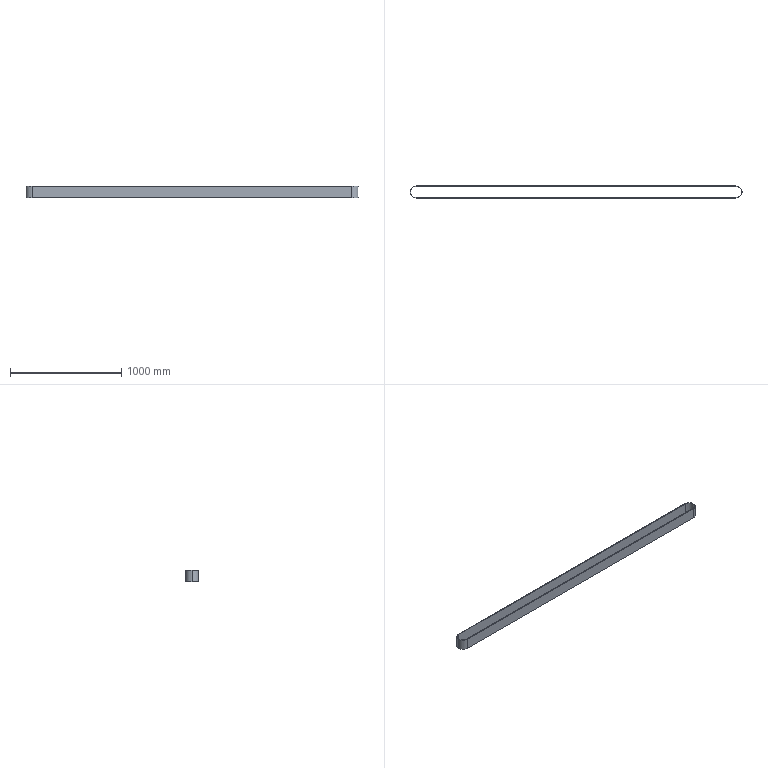Part | STEP file | 1 solid | 12 faces | box 2985 x 110 x 100 mm | volume 3039827 mm3 | cylinder 6 | plane 6 | commonest cylinder face diameters 100 x3 110 x3
STEP:
#1=CARTESIAN_POINT('',(0.,0.,0.));
#2=DIRECTION('',(0.,0.,1.));
#3=DIRECTION('',(1.,0.,0.));
#4=AXIS2_PLACEMENT_3D('',#1,#2,#3);
#5=CARTESIAN_POINT('',(-2874.893,50.,50.));
#6=VERTEX_POINT('',#5);
#7=CARTESIAN_POINT('',(-2874.893,50.,-50.));
#8=VERTEX_POINT('',#7);
#9=CARTESIAN_POINT('',(-2874.893,50.,50.));
#10=DIRECTION('',(0.,0.,-1.));
#11=VECTOR('',#10,1.);
#12=LINE('',#9,#11);
#13=CARTESIAN_POINT('',(-2874.893,0.,50.));
#14=DIRECTION('',(0.,0.,-1.));
#15=DIRECTION('',(-1.,0.,0.));
#16=AXIS2_PLACEMENT_3D('',#13,#14,#15);
#17=CYLINDRICAL_SURFACE('',#16,50.);
#18=CARTESIAN_POINT('',(1.571,0.));
#19=DIRECTION('',(0.,1.));
#20=VECTOR('',#19,1.);
#21=LINE('',#18,#20);
#22=(GEOMETRIC_REPRESENTATION_CONTEXT(2)PARAMETRIC_REPRESENTATION_CONTEXT()REPRESENTATION_CONTEXT('',''));
#23=DEFINITIONAL_REPRESENTATION('',(#21),#22);
#24=PCURVE('',#17,#23);
#25=CARTESIAN_POINT('',(-2874.893,50.,50.));
#26=DIRECTION('',(0.,1.,0.));
#27=DIRECTION('',(-1.,0.,0.));
#28=AXIS2_PLACEMENT_3D('',#25,#26,#27);
#29=PLANE('',#28);
#30=CARTESIAN_POINT('',(0.,0.));
#31=DIRECTION('',(0.,-1.));
#32=VECTOR('',#31,1.);
#33=LINE('',#30,#32);
#34=(GEOMETRIC_REPRESENTATION_CONTEXT(2)PARAMETRIC_REPRESENTATION_CONTEXT()REPRESENTATION_CONTEXT('',''));
#35=DEFINITIONAL_REPRESENTATION('',(#33),#34);
#36=PCURVE('',#29,#35);
#37=SURFACE_CURVE('',#12,(#24,#36),.PCURVE_S1.);
#38=EDGE_CURVE('',#6,#8,#37,.T.);
#39=ORIENTED_EDGE('',*,*,#38,.T.);
#40=CARTESIAN_POINT('',(-2924.893,0.,-50.));
#41=VERTEX_POINT('',#40);
#42=CARTESIAN_POINT('',(-2874.893,0.,-50.));
#43=DIRECTION('',(0.,0.,-1.));
#44=DIRECTION('',(-1.,0.,0.));
#45=AXIS2_PLACEMENT_3D('',#42,#43,#44);
#46=CIRCLE('',#45,50.);
#47=CARTESIAN_POINT('',(0.,100.));
#48=DIRECTION('',(1.,0.));
#49=VECTOR('',#48,1.);
#50=LINE('',#47,#49);
#51=(GEOMETRIC_REPRESENTATION_CONTEXT(2)PARAMETRIC_REPRESENTATION_CONTEXT()REPRESENTATION_CONTEXT('',''));
#52=DEFINITIONAL_REPRESENTATION('',(#50),#51);
#53=PCURVE('',#17,#52);
#54=CARTESIAN_POINT('',(-2874.893,0.,-50.));
#55=DIRECTION('',(0.,0.,-1.));
#56=DIRECTION('',(-1.,0.,0.));
#57=AXIS2_PLACEMENT_3D('',#54,#55,#56);
#58=PLANE('',#57);
#59=CARTESIAN_POINT('',(0.,0.));
#60=DIRECTION('',(1.,0.));
#61=AXIS2_PLACEMENT_2D('',#59,#60);
#62=CIRCLE('',#61,50.);
#63=(GEOMETRIC_REPRESENTATION_CONTEXT(2)PARAMETRIC_REPRESENTATION_CONTEXT()REPRESENTATION_CONTEXT('',''));
#64=DEFINITIONAL_REPRESENTATION('',(#62),#63);
#65=PCURVE('',#58,#64);
#66=SURFACE_CURVE('',#46,(#53,#65),.PCURVE_S1.);
#67=EDGE_CURVE('',#41,#8,#66,.T.);
#68=ORIENTED_EDGE('',*,*,#67,.F.);
#69=CARTESIAN_POINT('',(-2924.893,0.,50.));
#70=VERTEX_POINT('',#69);
#71=CARTESIAN_POINT('',(-2924.893,0.,50.));
#72=DIRECTION('',(0.,0.,-1.));
#73=VECTOR('',#72,1.);
#74=LINE('',#71,#73);
#75=CARTESIAN_POINT('',(0.,0.));
#76=DIRECTION('',(0.,1.));
#77=VECTOR('',#76,1.);
#78=LINE('',#75,#77);
#79=(GEOMETRIC_REPRESENTATION_CONTEXT(2)PARAMETRIC_REPRESENTATION_CONTEXT()REPRESENTATION_CONTEXT('',''));
#80=DEFINITIONAL_REPRESENTATION('',(#78),#79);
#81=PCURVE('',#17,#80);
#82=CARTESIAN_POINT('',(-2874.893,0.,50.));
#83=DIRECTION('',(0.,0.,-1.));
#84=DIRECTION('',(-1.,0.,0.));
#85=AXIS2_PLACEMENT_3D('',#82,#83,#84);
#86=CYLINDRICAL_SURFACE('',#85,50.);
#87=CARTESIAN_POINT('',(6.283,0.));
#88=DIRECTION('',(0.,1.));
#89=VECTOR('',#88,1.);
#90=LINE('',#87,#89);
#91=(GEOMETRIC_REPRESENTATION_CONTEXT(2)PARAMETRIC_REPRESENTATION_CONTEXT()REPRESENTATION_CONTEXT('',''));
#92=DEFINITIONAL_REPRESENTATION('',(#90),#91);
#93=PCURVE('',#86,#92);
#94=SURFACE_CURVE('',#74,(#81,#93),.PCURVE_S1.);
#95=EDGE_CURVE('',#70,#41,#94,.T.);
#96=ORIENTED_EDGE('',*,*,#95,.F.);
#97=CARTESIAN_POINT('',(-2874.893,0.,50.));
#98=DIRECTION('',(0.,0.,-1.));
#99=DIRECTION('',(-1.,0.,0.));
#100=AXIS2_PLACEMENT_3D('',#97,#98,#99);
#101=CIRCLE('',#100,50.);
#102=CARTESIAN_POINT('',(0.,0.));
#103=DIRECTION('',(1.,0.));
#104=VECTOR('',#103,1.);
#105=LINE('',#102,#104);
#106=(GEOMETRIC_REPRESENTATION_CONTEXT(2)PARAMETRIC_REPRESENTATION_CONTEXT()REPRESENTATION_CONTEXT('',''));
#107=DEFINITIONAL_REPRESENTATION('',(#105),#106);
#108=PCURVE('',#17,#107);
#109=CARTESIAN_POINT('',(-2874.893,0.,50.));
#110=DIRECTION('',(0.,0.,-1.));
#111=DIRECTION('',(-1.,0.,0.));
#112=AXIS2_PLACEMENT_3D('',#109,#110,#111);
#113=PLANE('',#112);
#114=CARTESIAN_POINT('',(0.,0.));
#115=DIRECTION('',(1.,0.));
#116=AXIS2_PLACEMENT_2D('',#114,#115);
#117=CIRCLE('',#116,50.);
#118=(GEOMETRIC_REPRESENTATION_CONTEXT(2)PARAMETRIC_REPRESENTATION_CONTEXT()REPRESENTATION_CONTEXT('',''));
#119=DEFINITIONAL_REPRESENTATION('',(#117),#118);
#120=PCURVE('',#113,#119);
#121=SURFACE_CURVE('',#101,(#108,#120),.PCURVE_S1.);
#122=EDGE_CURVE('',#70,#6,#121,.T.);
#123=ORIENTED_EDGE('',*,*,#122,.T.);
#124=EDGE_LOOP('',(#39,#68,#96,#123));
#125=FACE_BOUND('',#124,.F.);
#126=ADVANCED_FACE('',(#125),#17,.F.);
#127=CARTESIAN_POINT('',(-2874.893,-55.,50.));
#128=VERTEX_POINT('',#127);
#129=CARTESIAN_POINT('',(-2929.893,0.,50.));
#130=VERTEX_POINT('',#129);
#131=CARTESIAN_POINT('',(-2874.893,0.,50.));
#132=DIRECTION('',(0.,0.,-1.));
#133=DIRECTION('',(-1.,0.,0.));
#134=AXIS2_PLACEMENT_3D('',#131,#132,#133);
#135=CIRCLE('',#134,55.);
#136=CARTESIAN_POINT('',(-2874.893,0.,50.));
#137=DIRECTION('',(0.,0.,-1.));
#138=DIRECTION('',(-1.,0.,0.));
#139=AXIS2_PLACEMENT_3D('',#136,#137,#138);
#140=CYLINDRICAL_SURFACE('',#139,55.);
#141=CARTESIAN_POINT('',(0.,0.));
#142=DIRECTION('',(1.,0.));
#143=VECTOR('',#142,1.);
#144=LINE('',#141,#143);
#145=(GEOMETRIC_REPRESENTATION_CONTEXT(2)PARAMETRIC_REPRESENTATION_CONTEXT()REPRESENTATION_CONTEXT('',''));
#146=DEFINITIONAL_REPRESENTATION('',(#144),#145);
#147=PCURVE('',#140,#146);
#148=CARTESIAN_POINT('',(0.,0.));
#149=DIRECTION('',(1.,0.));
#150=AXIS2_PLACEMENT_2D('',#148,#149);
#151=CIRCLE('',#150,55.);
#152=(GEOMETRIC_REPRESENTATION_CONTEXT(2)PARAMETRIC_REPRESENTATION_CONTEXT()REPRESENTATION_CONTEXT('',''));
#153=DEFINITIONAL_REPRESENTATION('',(#151),#152);
#154=PCURVE('',#113,#153);
#155=SURFACE_CURVE('',#135,(#147,#154),.PCURVE_S1.);
#156=EDGE_CURVE('',#128,#130,#155,.T.);
#157=ORIENTED_EDGE('',*,*,#156,.T.);
#158=CARTESIAN_POINT('',(-2929.893,0.,-50.));
#159=VERTEX_POINT('',#158);
#160=CARTESIAN_POINT('',(-2929.893,0.,50.));
#161=DIRECTION('',(0.,0.,-1.));
#162=VECTOR('',#161,1.);
#163=LINE('',#160,#162);
#164=CARTESIAN_POINT('',(6.283,0.));
#165=DIRECTION('',(0.,1.));
#166=VECTOR('',#165,1.);
#167=LINE('',#164,#166);
#168=(GEOMETRIC_REPRESENTATION_CONTEXT(2)PARAMETRIC_REPRESENTATION_CONTEXT()REPRESENTATION_CONTEXT('',''));
#169=DEFINITIONAL_REPRESENTATION('',(#167),#168);
#170=PCURVE('',#140,#169);
#171=CARTESIAN_POINT('',(-2874.893,0.,50.));
#172=DIRECTION('',(0.,0.,-1.));
#173=DIRECTION('',(-1.,0.,0.));
#174=AXIS2_PLACEMENT_3D('',#171,#172,#173);
#175=CYLINDRICAL_SURFACE('',#174,55.);
#176=CARTESIAN_POINT('',(0.,0.));
#177=DIRECTION('',(0.,1.));
#178=VECTOR('',#177,1.);
#179=LINE('',#176,#178);
#180=(GEOMETRIC_REPRESENTATION_CONTEXT(2)PARAMETRIC_REPRESENTATION_CONTEXT()REPRESENTATION_CONTEXT('',''));
#181=DEFINITIONAL_REPRESENTATION('',(#179),#180);
#182=PCURVE('',#175,#181);
#183=SURFACE_CURVE('',#163,(#170,#182),.PCURVE_S1.);
#184=EDGE_CURVE('',#130,#159,#183,.T.);
#185=ORIENTED_EDGE('',*,*,#184,.T.);
#186=CARTESIAN_POINT('',(-2874.893,-55.,-50.));
#187=VERTEX_POINT('',#186);
#188=CARTESIAN_POINT('',(-2874.893,0.,-50.));
#189=DIRECTION('',(0.,0.,-1.));
#190=DIRECTION('',(-1.,0.,0.));
#191=AXIS2_PLACEMENT_3D('',#188,#189,#190);
#192=CIRCLE('',#191,55.);
#193=CARTESIAN_POINT('',(0.,100.));
#194=DIRECTION('',(1.,0.));
#195=VECTOR('',#194,1.);
#196=LINE('',#193,#195);
#197=(GEOMETRIC_REPRESENTATION_CONTEXT(2)PARAMETRIC_REPRESENTATION_CONTEXT()REPRESENTATION_CONTEXT('',''));
#198=DEFINITIONAL_REPRESENTATION('',(#196),#197);
#199=PCURVE('',#140,#198);
#200=CARTESIAN_POINT('',(0.,0.));
#201=DIRECTION('',(1.,0.));
#202=AXIS2_PLACEMENT_2D('',#200,#201);
#203=CIRCLE('',#202,55.);
#204=(GEOMETRIC_REPRESENTATION_CONTEXT(2)PARAMETRIC_REPRESENTATION_CONTEXT()REPRESENTATION_CONTEXT('',''));
#205=DEFINITIONAL_REPRESENTATION('',(#203),#204);
#206=PCURVE('',#58,#205);
#207=SURFACE_CURVE('',#192,(#199,#206),.PCURVE_S1.);
#208=EDGE_CURVE('',#187,#159,#207,.T.);
#209=ORIENTED_EDGE('',*,*,#208,.F.);
#210=CARTESIAN_POINT('',(-2874.893,-55.,50.));
#211=DIRECTION('',(0.,0.,-1.));
#212=VECTOR('',#211,1.);
#213=LINE('',#210,#212);
#214=CARTESIAN_POINT('',(4.712,0.));
#215=DIRECTION('',(0.,1.));
#216=VECTOR('',#215,1.);
#217=LINE('',#214,#216);
#218=(GEOMETRIC_REPRESENTATION_CONTEXT(2)PARAMETRIC_REPRESENTATION_CONTEXT()REPRESENTATION_CONTEXT('',''));
#219=DEFINITIONAL_REPRESENTATION('',(#217),#218);
#220=PCURVE('',#140,#219);
#221=CARTESIAN_POINT('',(-2874.893,-55.,50.));
#222=DIRECTION('',(0.,-1.,0.));
#223=DIRECTION('',(1.,0.,0.));
#224=AXIS2_PLACEMENT_3D('',#221,#222,#223);
#225=PLANE('',#224);
#226=CARTESIAN_POINT('',(0.,0.));
#227=DIRECTION('',(0.,-1.));
#228=VECTOR('',#227,1.);
#229=LINE('',#226,#228);
#230=(GEOMETRIC_REPRESENTATION_CONTEXT(2)PARAMETRIC_REPRESENTATION_CONTEXT()REPRESENTATION_CONTEXT('',''));
#231=DEFINITIONAL_REPRESENTATION('',(#229),#230);
#232=PCURVE('',#225,#231);
#233=SURFACE_CURVE('',#213,(#220,#232),.PCURVE_S1.);
#234=EDGE_CURVE('',#128,#187,#233,.T.);
#235=ORIENTED_EDGE('',*,*,#234,.F.);
#236=EDGE_LOOP('',(#157,#185,#209,#235));
#237=FACE_BOUND('',#236,.T.);
#238=ADVANCED_FACE('',(#237),#140,.T.);
#239=CARTESIAN_POINT('',(0.,-55.,-50.));
#240=VERTEX_POINT('',#239);
#241=CARTESIAN_POINT('',(-2874.893,-55.,-50.));
#242=DIRECTION('',(-1.,0.,0.));
#243=VECTOR('',#242,1.);
#244=LINE('',#241,#243);
#245=CARTESIAN_POINT('',(0.,-100.));
#246=DIRECTION('',(-1.,0.));
#247=VECTOR('',#246,1.);
#248=LINE('',#245,#247);
#249=(GEOMETRIC_REPRESENTATION_CONTEXT(2)PARAMETRIC_REPRESENTATION_CONTEXT()REPRESENTATION_CONTEXT('',''));
#250=DEFINITIONAL_REPRESENTATION('',(#248),#249);
#251=PCURVE('',#225,#250);
#252=CARTESIAN_POINT('',(0.,-55.));
#253=DIRECTION('',(1.,0.));
#254=VECTOR('',#253,1.);
#255=LINE('',#252,#254);
#256=(GEOMETRIC_REPRESENTATION_CONTEXT(2)PARAMETRIC_REPRESENTATION_CONTEXT()REPRESENTATION_CONTEXT('',''));
#257=DEFINITIONAL_REPRESENTATION('',(#255),#256);
#258=PCURVE('',#58,#257);
#259=SURFACE_CURVE('',#244,(#251,#258),.PCURVE_S1.);
#260=EDGE_CURVE('',#240,#187,#259,.T.);
#261=ORIENTED_EDGE('',*,*,#260,.F.);
#262=CARTESIAN_POINT('',(0.,-55.,50.));
#263=VERTEX_POINT('',#262);
#264=CARTESIAN_POINT('',(0.,-55.,50.));
#265=DIRECTION('',(0.,0.,-1.));
#266=VECTOR('',#265,1.);
#267=LINE('',#264,#266);
#268=CARTESIAN_POINT('',(2874.893,0.));
#269=DIRECTION('',(0.,-1.));
#270=VECTOR('',#269,1.);
#271=LINE('',#268,#270);
#272=(GEOMETRIC_REPRESENTATION_CONTEXT(2)PARAMETRIC_REPRESENTATION_CONTEXT()REPRESENTATION_CONTEXT('',''));
#273=DEFINITIONAL_REPRESENTATION('',(#271),#272);
#274=PCURVE('',#225,#273);
#275=CARTESIAN_POINT('',(0.,0.,50.));
#276=DIRECTION('',(0.,0.,-1.));
#277=DIRECTION('',(-1.,0.,0.));
#278=AXIS2_PLACEMENT_3D('',#275,#276,#277);
#279=CYLINDRICAL_SURFACE('',#278,55.);
#280=CARTESIAN_POINT('',(4.712,0.));
#281=DIRECTION('',(0.,1.));
#282=VECTOR('',#281,1.);
#283=LINE('',#280,#282);
#284=(GEOMETRIC_REPRESENTATION_CONTEXT(2)PARAMETRIC_REPRESENTATION_CONTEXT()REPRESENTATION_CONTEXT('',''));
#285=DEFINITIONAL_REPRESENTATION('',(#283),#284);
#286=PCURVE('',#279,#285);
#287=SURFACE_CURVE('',#267,(#274,#286),.PCURVE_S1.);
#288=EDGE_CURVE('',#263,#240,#287,.T.);
#289=ORIENTED_EDGE('',*,*,#288,.F.);
#290=CARTESIAN_POINT('',(-2874.893,-55.,50.));
#291=DIRECTION('',(-1.,0.,0.));
#292=VECTOR('',#291,1.);
#293=LINE('',#290,#292);
#294=CARTESIAN_POINT('',(0.,0.));
#295=DIRECTION('',(-1.,0.));
#296=VECTOR('',#295,1.);
#297=LINE('',#294,#296);
#298=(GEOMETRIC_REPRESENTATION_CONTEXT(2)PARAMETRIC_REPRESENTATION_CONTEXT()REPRESENTATION_CONTEXT('',''));
#299=DEFINITIONAL_REPRESENTATION('',(#297),#298);
#300=PCURVE('',#225,#299);
#301=CARTESIAN_POINT('',(0.,-55.));
#302=DIRECTION('',(1.,0.));
#303=VECTOR('',#302,1.);
#304=LINE('',#301,#303);
#305=(GEOMETRIC_REPRESENTATION_CONTEXT(2)PARAMETRIC_REPRESENTATION_CONTEXT()REPRESENTATION_CONTEXT('',''));
#306=DEFINITIONAL_REPRESENTATION('',(#304),#305);
#307=PCURVE('',#113,#306);
#308=SURFACE_CURVE('',#293,(#300,#307),.PCURVE_S1.);
#309=EDGE_CURVE('',#263,#128,#308,.T.);
#310=ORIENTED_EDGE('',*,*,#309,.T.);
#311=ORIENTED_EDGE('',*,*,#234,.T.);
#312=EDGE_LOOP('',(#261,#289,#310,#311));
#313=FACE_BOUND('',#312,.T.);
#314=ADVANCED_FACE('',(#313),#225,.T.);
#315=CARTESIAN_POINT('',(0.,55.,-50.));
#316=VERTEX_POINT('',#315);
#317=CARTESIAN_POINT('',(0.,0.,-50.));
#318=DIRECTION('',(0.,0.,-1.));
#319=DIRECTION('',(-1.,0.,0.));
#320=AXIS2_PLACEMENT_3D('',#317,#318,#319);
#321=CIRCLE('',#320,55.);
#322=CARTESIAN_POINT('',(0.,100.));
#323=DIRECTION('',(1.,0.));
#324=VECTOR('',#323,1.);
#325=LINE('',#322,#324);
#326=(GEOMETRIC_REPRESENTATION_CONTEXT(2)PARAMETRIC_REPRESENTATION_CONTEXT()REPRESENTATION_CONTEXT('',''));
#327=DEFINITIONAL_REPRESENTATION('',(#325),#326);
#328=PCURVE('',#279,#327);
#329=CARTESIAN_POINT('',(-2874.893,0.));
#330=DIRECTION('',(1.,0.));
#331=AXIS2_PLACEMENT_2D('',#329,#330);
#332=CIRCLE('',#331,55.);
#333=(GEOMETRIC_REPRESENTATION_CONTEXT(2)PARAMETRIC_REPRESENTATION_CONTEXT()REPRESENTATION_CONTEXT('',''));
#334=DEFINITIONAL_REPRESENTATION('',(#332),#333);
#335=PCURVE('',#58,#334);
#336=SURFACE_CURVE('',#321,(#328,#335),.PCURVE_S1.);
#337=EDGE_CURVE('',#316,#240,#336,.T.);
#338=ORIENTED_EDGE('',*,*,#337,.F.);
#339=CARTESIAN_POINT('',(0.,55.,50.));
#340=VERTEX_POINT('',#339);
#341=CARTESIAN_POINT('',(0.,55.,50.));
#342=DIRECTION('',(0.,0.,-1.));
#343=VECTOR('',#342,1.);
#344=LINE('',#341,#343);
#345=CARTESIAN_POINT('',(1.571,0.));
#346=DIRECTION('',(0.,1.));
#347=VECTOR('',#346,1.);
#348=LINE('',#345,#347);
#349=(GEOMETRIC_REPRESENTATION_CONTEXT(2)PARAMETRIC_REPRESENTATION_CONTEXT()REPRESENTATION_CONTEXT('',''));
#350=DEFINITIONAL_REPRESENTATION('',(#348),#349);
#351=PCURVE('',#279,#350);
#352=CARTESIAN_POINT('',(-2874.893,55.,50.));
#353=DIRECTION('',(0.,1.,0.));
#354=DIRECTION('',(-1.,0.,0.));
#355=AXIS2_PLACEMENT_3D('',#352,#353,#354);
#356=PLANE('',#355);
#357=CARTESIAN_POINT('',(-2874.893,0.));
#358=DIRECTION('',(0.,-1.));
#359=VECTOR('',#358,1.);
#360=LINE('',#357,#359);
#361=(GEOMETRIC_REPRESENTATION_CONTEXT(2)PARAMETRIC_REPRESENTATION_CONTEXT()REPRESENTATION_CONTEXT('',''));
#362=DEFINITIONAL_REPRESENTATION('',(#360),#361);
#363=PCURVE('',#356,#362);
#364=SURFACE_CURVE('',#344,(#351,#363),.PCURVE_S1.);
#365=EDGE_CURVE('',#340,#316,#364,.T.);
#366=ORIENTED_EDGE('',*,*,#365,.F.);
#367=CARTESIAN_POINT('',(0.,0.,50.));
#368=DIRECTION('',(0.,0.,-1.));
#369=DIRECTION('',(-1.,0.,0.));
#370=AXIS2_PLACEMENT_3D('',#367,#368,#369);
#371=CIRCLE('',#370,55.);
#372=CARTESIAN_POINT('',(0.,0.));
#373=DIRECTION('',(1.,0.));
#374=VECTOR('',#373,1.);
#375=LINE('',#372,#374);
#376=(GEOMETRIC_REPRESENTATION_CONTEXT(2)PARAMETRIC_REPRESENTATION_CONTEXT()REPRESENTATION_CONTEXT('',''));
#377=DEFINITIONAL_REPRESENTATION('',(#375),#376);
#378=PCURVE('',#279,#377);
#379=CARTESIAN_POINT('',(-2874.893,0.));
#380=DIRECTION('',(1.,0.));
#381=AXIS2_PLACEMENT_2D('',#379,#380);
#382=CIRCLE('',#381,55.);
#383=(GEOMETRIC_REPRESENTATION_CONTEXT(2)PARAMETRIC_REPRESENTATION_CONTEXT()REPRESENTATION_CONTEXT('',''));
#384=DEFINITIONAL_REPRESENTATION('',(#382),#383);
#385=PCURVE('',#113,#384);
#386=SURFACE_CURVE('',#371,(#378,#385),.PCURVE_S1.);
#387=EDGE_CURVE('',#340,#263,#386,.T.);
#388=ORIENTED_EDGE('',*,*,#387,.T.);
#389=ORIENTED_EDGE('',*,*,#288,.T.);
#390=EDGE_LOOP('',(#338,#366,#388,#389));
#391=FACE_BOUND('',#390,.T.);
#392=ADVANCED_FACE('',(#391),#279,.T.);
#393=CARTESIAN_POINT('',(-2874.893,55.,-50.));
#394=VERTEX_POINT('',#393);
#395=CARTESIAN_POINT('',(-2874.893,55.,-50.));
#396=DIRECTION('',(1.,0.,0.));
#397=VECTOR('',#396,1.);
#398=LINE('',#395,#397);
#399=CARTESIAN_POINT('',(0.,-100.));
#400=DIRECTION('',(-1.,0.));
#401=VECTOR('',#400,1.);
#402=LINE('',#399,#401);
#403=(GEOMETRIC_REPRESENTATION_CONTEXT(2)PARAMETRIC_REPRESENTATION_CONTEXT()REPRESENTATION_CONTEXT('',''));
#404=DEFINITIONAL_REPRESENTATION('',(#402),#403);
#405=PCURVE('',#356,#404);
#406=CARTESIAN_POINT('',(0.,55.));
#407=DIRECTION('',(-1.,0.));
#408=VECTOR('',#407,1.);
#409=LINE('',#406,#408);
#410=(GEOMETRIC_REPRESENTATION_CONTEXT(2)PARAMETRIC_REPRESENTATION_CONTEXT()REPRESENTATION_CONTEXT('',''));
#411=DEFINITIONAL_REPRESENTATION('',(#409),#410);
#412=PCURVE('',#58,#411);
#413=SURFACE_CURVE('',#398,(#405,#412),.PCURVE_S1.);
#414=EDGE_CURVE('',#394,#316,#413,.T.);
#415=ORIENTED_EDGE('',*,*,#414,.F.);
#416=CARTESIAN_POINT('',(-2874.893,55.,50.));
#417=VERTEX_POINT('',#416);
#418=CARTESIAN_POINT('',(-2874.893,55.,50.));
#419=DIRECTION('',(0.,0.,-1.));
#420=VECTOR('',#419,1.);
#421=LINE('',#418,#420);
#422=CARTESIAN_POINT('',(0.,0.));
#423=DIRECTION('',(0.,-1.));
#424=VECTOR('',#423,1.);
#425=LINE('',#422,#424);
#426=(GEOMETRIC_REPRESENTATION_CONTEXT(2)PARAMETRIC_REPRESENTATION_CONTEXT()REPRESENTATION_CONTEXT('',''));
#427=DEFINITIONAL_REPRESENTATION('',(#425),#426);
#428=PCURVE('',#356,#427);
#429=CARTESIAN_POINT('',(1.571,0.));
#430=DIRECTION('',(0.,1.));
#431=VECTOR('',#430,1.);
#432=LINE('',#429,#431);
#433=(GEOMETRIC_REPRESENTATION_CONTEXT(2)PARAMETRIC_REPRESENTATION_CONTEXT()REPRESENTATION_CONTEXT('',''));
#434=DEFINITIONAL_REPRESENTATION('',(#432),#433);
#435=PCURVE('',#175,#434);
#436=SURFACE_CURVE('',#421,(#428,#435),.PCURVE_S1.);
#437=EDGE_CURVE('',#417,#394,#436,.T.);
#438=ORIENTED_EDGE('',*,*,#437,.F.);
#439=CARTESIAN_POINT('',(-2874.893,55.,50.));
#440=DIRECTION('',(1.,0.,0.));
#441=VECTOR('',#440,1.);
#442=LINE('',#439,#441);
#443=CARTESIAN_POINT('',(0.,0.));
#444=DIRECTION('',(-1.,0.));
#445=VECTOR('',#444,1.);
#446=LINE('',#443,#445);
#447=(GEOMETRIC_REPRESENTATION_CONTEXT(2)PARAMETRIC_REPRESENTATION_CONTEXT()REPRESENTATION_CONTEXT('',''));
#448=DEFINITIONAL_REPRESENTATION('',(#446),#447);
#449=PCURVE('',#356,#448);
#450=CARTESIAN_POINT('',(0.,55.));
#451=DIRECTION('',(-1.,0.));
#452=VECTOR('',#451,1.);
#453=LINE('',#450,#452);
#454=(GEOMETRIC_REPRESENTATION_CONTEXT(2)PARAMETRIC_REPRESENTATION_CONTEXT()REPRESENTATION_CONTEXT('',''));
#455=DEFINITIONAL_REPRESENTATION('',(#453),#454);
#456=PCURVE('',#113,#455);
#457=SURFACE_CURVE('',#442,(#449,#456),.PCURVE_S1.);
#458=EDGE_CURVE('',#417,#340,#457,.T.);
#459=ORIENTED_EDGE('',*,*,#458,.T.);
#460=ORIENTED_EDGE('',*,*,#365,.T.);
#461=EDGE_LOOP('',(#415,#438,#459,#460));
#462=FACE_BOUND('',#461,.T.);
#463=ADVANCED_FACE('',(#462),#356,.T.);
#464=ORIENTED_EDGE('',*,*,#184,.F.);
#465=CARTESIAN_POINT('',(-2874.893,0.,50.));
#466=DIRECTION('',(0.,0.,-1.));
#467=DIRECTION('',(-1.,0.,0.));
#468=AXIS2_PLACEMENT_3D('',#465,#466,#467);
#469=CIRCLE('',#468,55.);
#470=CARTESIAN_POINT('',(0.,0.));
#471=DIRECTION('',(1.,0.));
#472=VECTOR('',#471,1.);
#473=LINE('',#470,#472);
#474=(GEOMETRIC_REPRESENTATION_CONTEXT(2)PARAMETRIC_REPRESENTATION_CONTEXT()REPRESENTATION_CONTEXT('',''));
#475=DEFINITIONAL_REPRESENTATION('',(#473),#474);
#476=PCURVE('',#175,#475);
#477=CARTESIAN_POINT('',(0.,0.));
#478=DIRECTION('',(1.,0.));
#479=AXIS2_PLACEMENT_2D('',#477,#478);
#480=CIRCLE('',#479,55.);
#481=(GEOMETRIC_REPRESENTATION_CONTEXT(2)PARAMETRIC_REPRESENTATION_CONTEXT()REPRESENTATION_CONTEXT('',''));
#482=DEFINITIONAL_REPRESENTATION('',(#480),#481);
#483=PCURVE('',#113,#482);
#484=SURFACE_CURVE('',#469,(#476,#483),.PCURVE_S1.);
#485=EDGE_CURVE('',#130,#417,#484,.T.);
#486=ORIENTED_EDGE('',*,*,#485,.T.);
#487=ORIENTED_EDGE('',*,*,#437,.T.);
#488=CARTESIAN_POINT('',(-2874.893,0.,-50.));
#489=DIRECTION('',(0.,0.,-1.));
#490=DIRECTION('',(-1.,0.,0.));
#491=AXIS2_PLACEMENT_3D('',#488,#489,#490);
#492=CIRCLE('',#491,55.);
#493=CARTESIAN_POINT('',(0.,100.));
#494=DIRECTION('',(1.,0.));
#495=VECTOR('',#494,1.);
#496=LINE('',#493,#495);
#497=(GEOMETRIC_REPRESENTATION_CONTEXT(2)PARAMETRIC_REPRESENTATION_CONTEXT()REPRESENTATION_CONTEXT('',''));
#498=DEFINITIONAL_REPRESENTATION('',(#496),#497);
#499=PCURVE('',#175,#498);
#500=CARTESIAN_POINT('',(0.,0.));
#501=DIRECTION('',(1.,0.));
#502=AXIS2_PLACEMENT_2D('',#500,#501);
#503=CIRCLE('',#502,55.);
#504=(GEOMETRIC_REPRESENTATION_CONTEXT(2)PARAMETRIC_REPRESENTATION_CONTEXT()REPRESENTATION_CONTEXT('',''));
#505=DEFINITIONAL_REPRESENTATION('',(#503),#504);
#506=PCURVE('',#58,#505);
#507=SURFACE_CURVE('',#492,(#499,#506),.PCURVE_S1.);
#508=EDGE_CURVE('',#159,#394,#507,.T.);
#509=ORIENTED_EDGE('',*,*,#508,.F.);
#510=EDGE_LOOP('',(#464,#486,#487,#509));
#511=FACE_BOUND('',#510,.T.);
#512=ADVANCED_FACE('',(#511),#175,.T.);
#513=CARTESIAN_POINT('',(0.,50.,50.));
#514=VERTEX_POINT('',#513);
#515=CARTESIAN_POINT('',(0.,-50.,50.));
#516=VERTEX_POINT('',#515);
#517=CARTESIAN_POINT('',(0.,0.,50.));
#518=DIRECTION('',(0.,0.,-1.));
#519=DIRECTION('',(-1.,0.,0.));
#520=AXIS2_PLACEMENT_3D('',#517,#518,#519);
#521=CIRCLE('',#520,50.);
#522=CARTESIAN_POINT('',(-2874.893,0.));
#523=DIRECTION('',(1.,0.));
#524=AXIS2_PLACEMENT_2D('',#522,#523);
#525=CIRCLE('',#524,50.);
#526=(GEOMETRIC_REPRESENTATION_CONTEXT(2)PARAMETRIC_REPRESENTATION_CONTEXT()REPRESENTATION_CONTEXT('',''));
#527=DEFINITIONAL_REPRESENTATION('',(#525),#526);
#528=PCURVE('',#113,#527);
#529=CARTESIAN_POINT('',(0.,0.,50.));
#530=DIRECTION('',(0.,0.,-1.));
#531=DIRECTION('',(-1.,0.,0.));
#532=AXIS2_PLACEMENT_3D('',#529,#530,#531);
#533=CYLINDRICAL_SURFACE('',#532,50.);
#534=CARTESIAN_POINT('',(0.,0.));
#535=DIRECTION('',(1.,0.));
#536=VECTOR('',#535,1.);
#537=LINE('',#534,#536);
#538=(GEOMETRIC_REPRESENTATION_CONTEXT(2)PARAMETRIC_REPRESENTATION_CONTEXT()REPRESENTATION_CONTEXT('',''));
#539=DEFINITIONAL_REPRESENTATION('',(#537),#538);
#540=PCURVE('',#533,#539);
#541=SURFACE_CURVE('',#521,(#528,#540),.PCURVE_S1.);
#542=EDGE_CURVE('',#514,#516,#541,.T.);
#543=ORIENTED_EDGE('',*,*,#542,.T.);
#544=CARTESIAN_POINT('',(-2874.893,-50.,50.));
#545=VERTEX_POINT('',#544);
#546=CARTESIAN_POINT('',(0.,-50.,50.));
#547=DIRECTION('',(-1.,0.,0.));
#548=VECTOR('',#547,1.);
#549=LINE('',#546,#548);
#550=CARTESIAN_POINT('',(-2874.893,-50.));
#551=DIRECTION('',(1.,0.));
#552=VECTOR('',#551,1.);
#553=LINE('',#550,#552);
#554=(GEOMETRIC_REPRESENTATION_CONTEXT(2)PARAMETRIC_REPRESENTATION_CONTEXT()REPRESENTATION_CONTEXT('',''));
#555=DEFINITIONAL_REPRESENTATION('',(#553),#554);
#556=PCURVE('',#113,#555);
#557=CARTESIAN_POINT('',(0.,-50.,50.));
#558=DIRECTION('',(0.,-1.,0.));
#559=DIRECTION('',(1.,0.,0.));
#560=AXIS2_PLACEMENT_3D('',#557,#558,#559);
#561=PLANE('',#560);
#562=CARTESIAN_POINT('',(0.,0.));
#563=DIRECTION('',(-1.,0.));
#564=VECTOR('',#563,1.);
#565=LINE('',#562,#564);
#566=(GEOMETRIC_REPRESENTATION_CONTEXT(2)PARAMETRIC_REPRESENTATION_CONTEXT()REPRESENTATION_CONTEXT('',''));
#567=DEFINITIONAL_REPRESENTATION('',(#565),#566);
#568=PCURVE('',#561,#567);
#569=SURFACE_CURVE('',#549,(#556,#568),.PCURVE_S1.);
#570=EDGE_CURVE('',#516,#545,#569,.T.);
#571=ORIENTED_EDGE('',*,*,#570,.T.);
#572=CARTESIAN_POINT('',(-2874.893,0.,50.));
#573=DIRECTION('',(0.,0.,-1.));
#574=DIRECTION('',(-1.,0.,0.));
#575=AXIS2_PLACEMENT_3D('',#572,#573,#574);
#576=CIRCLE('',#575,50.);
#577=CARTESIAN_POINT('',(0.,0.));
#578=DIRECTION('',(1.,0.));
#579=AXIS2_PLACEMENT_2D('',#577,#578);
#580=CIRCLE('',#579,50.);
#581=(GEOMETRIC_REPRESENTATION_CONTEXT(2)PARAMETRIC_REPRESENTATION_CONTEXT()REPRESENTATION_CONTEXT('',''));
#582=DEFINITIONAL_REPRESENTATION('',(#580),#581);
#583=PCURVE('',#113,#582);
#584=CARTESIAN_POINT('',(0.,0.));
#585=DIRECTION('',(1.,0.));
#586=VECTOR('',#585,1.);
#587=LINE('',#584,#586);
#588=(GEOMETRIC_REPRESENTATION_CONTEXT(2)PARAMETRIC_REPRESENTATION_CONTEXT()REPRESENTATION_CONTEXT('',''));
#589=DEFINITIONAL_REPRESENTATION('',(#587),#588);
#590=PCURVE('',#86,#589);
#591=SURFACE_CURVE('',#576,(#583,#590),.PCURVE_S1.);
#592=EDGE_CURVE('',#545,#70,#591,.T.);
#593=ORIENTED_EDGE('',*,*,#592,.T.);
#594=ORIENTED_EDGE('',*,*,#122,.T.);
#595=CARTESIAN_POINT('',(-2874.893,50.,50.));
#596=DIRECTION('',(1.,0.,0.));
#597=VECTOR('',#596,1.);
#598=LINE('',#595,#597);
#599=CARTESIAN_POINT('',(0.,50.));
#600=DIRECTION('',(-1.,0.));
#601=VECTOR('',#600,1.);
#602=LINE('',#599,#601);
#603=(GEOMETRIC_REPRESENTATION_CONTEXT(2)PARAMETRIC_REPRESENTATION_CONTEXT()REPRESENTATION_CONTEXT('',''));
#604=DEFINITIONAL_REPRESENTATION('',(#602),#603);
#605=PCURVE('',#113,#604);
#606=CARTESIAN_POINT('',(0.,0.));
#607=DIRECTION('',(-1.,0.));
#608=VECTOR('',#607,1.);
#609=LINE('',#606,#608);
#610=(GEOMETRIC_REPRESENTATION_CONTEXT(2)PARAMETRIC_REPRESENTATION_CONTEXT()REPRESENTATION_CONTEXT('',''));
#611=DEFINITIONAL_REPRESENTATION('',(#609),#610);
#612=PCURVE('',#29,#611);
#613=SURFACE_CURVE('',#598,(#605,#612),.PCURVE_S1.);
#614=EDGE_CURVE('',#6,#514,#613,.T.);
#615=ORIENTED_EDGE('',*,*,#614,.T.);
#616=EDGE_LOOP('',(#543,#571,#593,#594,#615));
#617=FACE_BOUND('',#616,.T.);
#618=ORIENTED_EDGE('',*,*,#309,.F.);
#619=ORIENTED_EDGE('',*,*,#387,.F.);
#620=ORIENTED_EDGE('',*,*,#458,.F.);
#621=ORIENTED_EDGE('',*,*,#485,.F.);
#622=ORIENTED_EDGE('',*,*,#156,.F.);
#623=EDGE_LOOP('',(#618,#619,#620,#621,#622));
#624=FACE_BOUND('',#623,.T.);
#625=ADVANCED_FACE('',(#617,#624),#113,.F.);
#626=CARTESIAN_POINT('',(0.,-50.,-50.));
#627=VERTEX_POINT('',#626);
#628=CARTESIAN_POINT('',(-2874.893,-50.,-50.));
#629=VERTEX_POINT('',#628);
#630=CARTESIAN_POINT('',(0.,-50.,-50.));
#631=DIRECTION('',(-1.,0.,0.));
#632=VECTOR('',#631,1.);
#633=LINE('',#630,#632);
#634=CARTESIAN_POINT('',(-2874.893,-50.));
#635=DIRECTION('',(1.,0.));
#636=VECTOR('',#635,1.);
#637=LINE('',#634,#636);
#638=(GEOMETRIC_REPRESENTATION_CONTEXT(2)PARAMETRIC_REPRESENTATION_CONTEXT()REPRESENTATION_CONTEXT('',''));
#639=DEFINITIONAL_REPRESENTATION('',(#637),#638);
#640=PCURVE('',#58,#639);
#641=CARTESIAN_POINT('',(0.,-100.));
#642=DIRECTION('',(-1.,0.));
#643=VECTOR('',#642,1.);
#644=LINE('',#641,#643);
#645=(GEOMETRIC_REPRESENTATION_CONTEXT(2)PARAMETRIC_REPRESENTATION_CONTEXT()REPRESENTATION_CONTEXT('',''));
#646=DEFINITIONAL_REPRESENTATION('',(#644),#645);
#647=PCURVE('',#561,#646);
#648=SURFACE_CURVE('',#633,(#640,#647),.PCURVE_S1.);
#649=EDGE_CURVE('',#627,#629,#648,.T.);
#650=ORIENTED_EDGE('',*,*,#649,.F.);
#651=CARTESIAN_POINT('',(0.,50.,-50.));
#652=VERTEX_POINT('',#651);
#653=CARTESIAN_POINT('',(0.,0.,-50.));
#654=DIRECTION('',(0.,0.,-1.));
#655=DIRECTION('',(-1.,0.,0.));
#656=AXIS2_PLACEMENT_3D('',#653,#654,#655);
#657=CIRCLE('',#656,50.);
#658=CARTESIAN_POINT('',(-2874.893,0.));
#659=DIRECTION('',(1.,0.));
#660=AXIS2_PLACEMENT_2D('',#658,#659);
#661=CIRCLE('',#660,50.);
#662=(GEOMETRIC_REPRESENTATION_CONTEXT(2)PARAMETRIC_REPRESENTATION_CONTEXT()REPRESENTATION_CONTEXT('',''));
#663=DEFINITIONAL_REPRESENTATION('',(#661),#662);
#664=PCURVE('',#58,#663);
#665=CARTESIAN_POINT('',(0.,100.));
#666=DIRECTION('',(1.,0.));
#667=VECTOR('',#666,1.);
#668=LINE('',#665,#667);
#669=(GEOMETRIC_REPRESENTATION_CONTEXT(2)PARAMETRIC_REPRESENTATION_CONTEXT()REPRESENTATION_CONTEXT('',''));
#670=DEFINITIONAL_REPRESENTATION('',(#668),#669);
#671=PCURVE('',#533,#670);
#672=SURFACE_CURVE('',#657,(#664,#671),.PCURVE_S1.);
#673=EDGE_CURVE('',#652,#627,#672,.T.);
#674=ORIENTED_EDGE('',*,*,#673,.F.);
#675=CARTESIAN_POINT('',(-2874.893,50.,-50.));
#676=DIRECTION('',(1.,0.,0.));
#677=VECTOR('',#676,1.);
#678=LINE('',#675,#677);
#679=CARTESIAN_POINT('',(0.,50.));
#680=DIRECTION('',(-1.,0.));
#681=VECTOR('',#680,1.);
#682=LINE('',#679,#681);
#683=(GEOMETRIC_REPRESENTATION_CONTEXT(2)PARAMETRIC_REPRESENTATION_CONTEXT()REPRESENTATION_CONTEXT('',''));
#684=DEFINITIONAL_REPRESENTATION('',(#682),#683);
#685=PCURVE('',#58,#684);
#686=CARTESIAN_POINT('',(0.,-100.));
#687=DIRECTION('',(-1.,0.));
#688=VECTOR('',#687,1.);
#689=LINE('',#686,#688);
#690=(GEOMETRIC_REPRESENTATION_CONTEXT(2)PARAMETRIC_REPRESENTATION_CONTEXT()REPRESENTATION_CONTEXT('',''));
#691=DEFINITIONAL_REPRESENTATION('',(#689),#690);
#692=PCURVE('',#29,#691);
#693=SURFACE_CURVE('',#678,(#685,#692),.PCURVE_S1.);
#694=EDGE_CURVE('',#8,#652,#693,.T.);
#695=ORIENTED_EDGE('',*,*,#694,.F.);
#696=ORIENTED_EDGE('',*,*,#67,.F.);
#697=CARTESIAN_POINT('',(-2874.893,0.,-50.));
#698=DIRECTION('',(0.,0.,-1.));
#699=DIRECTION('',(-1.,0.,0.));
#700=AXIS2_PLACEMENT_3D('',#697,#698,#699);
#701=CIRCLE('',#700,50.);
#702=CARTESIAN_POINT('',(0.,0.));
#703=DIRECTION('',(1.,0.));
#704=AXIS2_PLACEMENT_2D('',#702,#703);
#705=CIRCLE('',#704,50.);
#706=(GEOMETRIC_REPRESENTATION_CONTEXT(2)PARAMETRIC_REPRESENTATION_CONTEXT()REPRESENTATION_CONTEXT('',''));
#707=DEFINITIONAL_REPRESENTATION('',(#705),#706);
#708=PCURVE('',#58,#707);
#709=CARTESIAN_POINT('',(0.,100.));
#710=DIRECTION('',(1.,0.));
#711=VECTOR('',#710,1.);
#712=LINE('',#709,#711);
#713=(GEOMETRIC_REPRESENTATION_CONTEXT(2)PARAMETRIC_REPRESENTATION_CONTEXT()REPRESENTATION_CONTEXT('',''));
#714=DEFINITIONAL_REPRESENTATION('',(#712),#713);
#715=PCURVE('',#86,#714);
#716=SURFACE_CURVE('',#701,(#708,#715),.PCURVE_S1.);
#717=EDGE_CURVE('',#629,#41,#716,.T.);
#718=ORIENTED_EDGE('',*,*,#717,.F.);
#719=EDGE_LOOP('',(#650,#674,#695,#696,#718));
#720=FACE_BOUND('',#719,.T.);
#721=ORIENTED_EDGE('',*,*,#260,.T.);
#722=ORIENTED_EDGE('',*,*,#208,.T.);
#723=ORIENTED_EDGE('',*,*,#508,.T.);
#724=ORIENTED_EDGE('',*,*,#414,.T.);
#725=ORIENTED_EDGE('',*,*,#337,.T.);
#726=EDGE_LOOP('',(#721,#722,#723,#724,#725));
#727=FACE_BOUND('',#726,.T.);
#728=ADVANCED_FACE('',(#720,#727),#58,.T.);
#729=ORIENTED_EDGE('',*,*,#649,.T.);
#730=CARTESIAN_POINT('',(-2874.893,-50.,50.));
#731=DIRECTION('',(0.,0.,-1.));
#732=VECTOR('',#731,1.);
#733=LINE('',#730,#732);
#734=CARTESIAN_POINT('',(-2874.893,0.));
#735=DIRECTION('',(0.,-1.));
#736=VECTOR('',#735,1.);
#737=LINE('',#734,#736);
#738=(GEOMETRIC_REPRESENTATION_CONTEXT(2)PARAMETRIC_REPRESENTATION_CONTEXT()REPRESENTATION_CONTEXT('',''));
#739=DEFINITIONAL_REPRESENTATION('',(#737),#738);
#740=PCURVE('',#561,#739);
#741=CARTESIAN_POINT('',(4.712,0.));
#742=DIRECTION('',(0.,1.));
#743=VECTOR('',#742,1.);
#744=LINE('',#741,#743);
#745=(GEOMETRIC_REPRESENTATION_CONTEXT(2)PARAMETRIC_REPRESENTATION_CONTEXT()REPRESENTATION_CONTEXT('',''));
#746=DEFINITIONAL_REPRESENTATION('',(#744),#745);
#747=PCURVE('',#86,#746);
#748=SURFACE_CURVE('',#733,(#740,#747),.PCURVE_S1.);
#749=EDGE_CURVE('',#545,#629,#748,.T.);
#750=ORIENTED_EDGE('',*,*,#749,.F.);
#751=ORIENTED_EDGE('',*,*,#570,.F.);
#752=CARTESIAN_POINT('',(0.,-50.,50.));
#753=DIRECTION('',(0.,0.,-1.));
#754=VECTOR('',#753,1.);
#755=LINE('',#752,#754);
#756=CARTESIAN_POINT('',(0.,0.));
#757=DIRECTION('',(0.,-1.));
#758=VECTOR('',#757,1.);
#759=LINE('',#756,#758);
#760=(GEOMETRIC_REPRESENTATION_CONTEXT(2)PARAMETRIC_REPRESENTATION_CONTEXT()REPRESENTATION_CONTEXT('',''));
#761=DEFINITIONAL_REPRESENTATION('',(#759),#760);
#762=PCURVE('',#561,#761);
#763=CARTESIAN_POINT('',(4.712,0.));
#764=DIRECTION('',(0.,1.));
#765=VECTOR('',#764,1.);
#766=LINE('',#763,#765);
#767=(GEOMETRIC_REPRESENTATION_CONTEXT(2)PARAMETRIC_REPRESENTATION_CONTEXT()REPRESENTATION_CONTEXT('',''));
#768=DEFINITIONAL_REPRESENTATION('',(#766),#767);
#769=PCURVE('',#533,#768);
#770=SURFACE_CURVE('',#755,(#762,#769),.PCURVE_S1.);
#771=EDGE_CURVE('',#516,#627,#770,.T.);
#772=ORIENTED_EDGE('',*,*,#771,.T.);
#773=EDGE_LOOP('',(#729,#750,#751,#772));
#774=FACE_BOUND('',#773,.T.);
#775=ADVANCED_FACE('',(#774),#561,.F.);
#776=CARTESIAN_POINT('',(0.,50.,50.));
#777=DIRECTION('',(0.,0.,-1.));
#778=VECTOR('',#777,1.);
#779=LINE('',#776,#778);
#780=CARTESIAN_POINT('',(1.571,0.));
#781=DIRECTION('',(0.,1.));
#782=VECTOR('',#781,1.);
#783=LINE('',#780,#782);
#784=(GEOMETRIC_REPRESENTATION_CONTEXT(2)PARAMETRIC_REPRESENTATION_CONTEXT()REPRESENTATION_CONTEXT('',''));
#785=DEFINITIONAL_REPRESENTATION('',(#783),#784);
#786=PCURVE('',#533,#785);
#787=CARTESIAN_POINT('',(-2874.893,0.));
#788=DIRECTION('',(0.,-1.));
#789=VECTOR('',#788,1.);
#790=LINE('',#787,#789);
#791=(GEOMETRIC_REPRESENTATION_CONTEXT(2)PARAMETRIC_REPRESENTATION_CONTEXT()REPRESENTATION_CONTEXT('',''));
#792=DEFINITIONAL_REPRESENTATION('',(#790),#791);
#793=PCURVE('',#29,#792);
#794=SURFACE_CURVE('',#779,(#786,#793),.PCURVE_S1.);
#795=EDGE_CURVE('',#514,#652,#794,.T.);
#796=ORIENTED_EDGE('',*,*,#795,.F.);
#797=ORIENTED_EDGE('',*,*,#542,.T.);
#798=ORIENTED_EDGE('',*,*,#771,.T.);
#799=ORIENTED_EDGE('',*,*,#673,.F.);
#800=EDGE_LOOP('',(#796,#797,#798,#799));
#801=FACE_BOUND('',#800,.F.);
#802=ADVANCED_FACE('',(#801),#533,.F.);
#803=ORIENTED_EDGE('',*,*,#694,.T.);
#804=ORIENTED_EDGE('',*,*,#795,.F.);
#805=ORIENTED_EDGE('',*,*,#614,.F.);
#806=ORIENTED_EDGE('',*,*,#38,.T.);
#807=EDGE_LOOP('',(#803,#804,#805,#806));
#808=FACE_BOUND('',#807,.T.);
#809=ADVANCED_FACE('',(#808),#29,.F.);
#810=ORIENTED_EDGE('',*,*,#717,.F.);
#811=ORIENTED_EDGE('',*,*,#749,.F.);
#812=ORIENTED_EDGE('',*,*,#592,.T.);
#813=ORIENTED_EDGE('',*,*,#95,.T.);
#814=EDGE_LOOP('',(#810,#811,#812,#813));
#815=FACE_BOUND('',#814,.F.);
#816=ADVANCED_FACE('',(#815),#86,.F.);
#817=CLOSED_SHELL('',(#126,#238,#314,#392,#463,#512,#625,#728,#775,#802,#809,#816));
#818=MANIFOLD_SOLID_BREP('',#817);
#819=(LENGTH_UNIT()NAMED_UNIT(*)SI_UNIT(.MILLI.,.METRE.));
#820=UNCERTAINTY_MEASURE_WITH_UNIT(LENGTH_MEASURE(0.0000001),#819,'','');
#821=(NAMED_UNIT(*)PLANE_ANGLE_UNIT()SI_UNIT($,.RADIAN.));
#822=(NAMED_UNIT(*)SI_UNIT($,.STERADIAN.)SOLID_ANGLE_UNIT());
#823=(GEOMETRIC_REPRESENTATION_CONTEXT(3)GLOBAL_UNCERTAINTY_ASSIGNED_CONTEXT((#820))GLOBAL_UNIT_ASSIGNED_CONTEXT((#819,#821,#822))REPRESENTATION_CONTEXT('',''));
#824=ADVANCED_BREP_SHAPE_REPRESENTATION('',(#4,#818),#823);